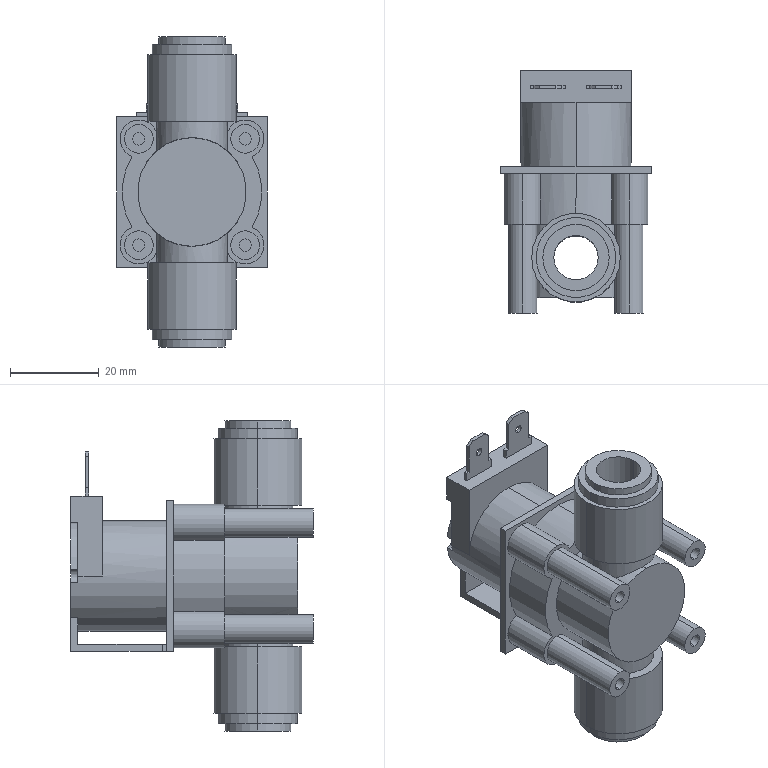Part | SolidWorks | features MBimport 1 | 1 solid | 124 faces | box 34 x 54.7 x 70 mm | volume 42821 mm3 | plane 64 | cylinder 60 | commonest cylinder face diameters 2.8 x8 6.5 x8 8.5 x6 31.5 x5 1.7 x4 3 x4